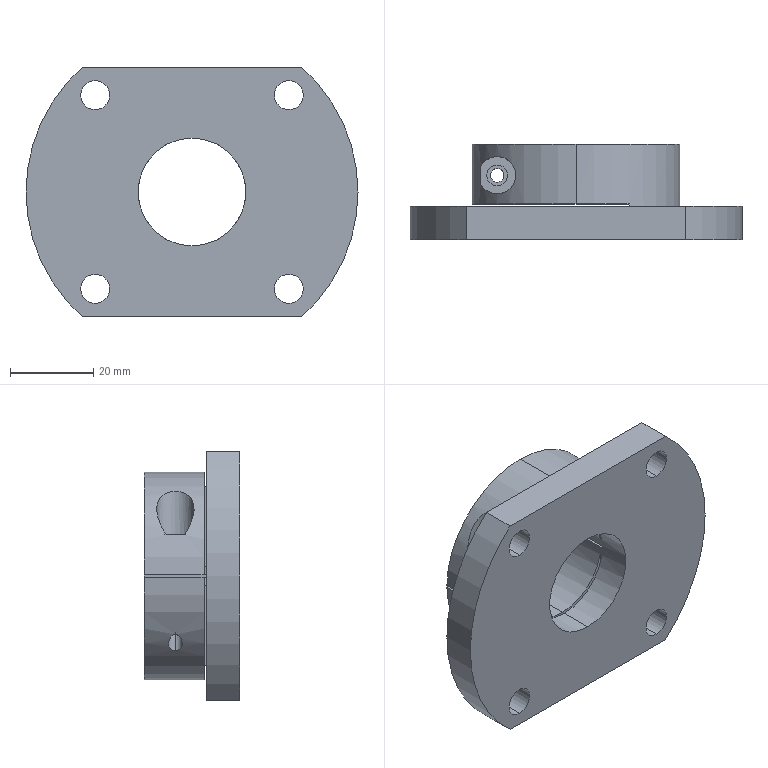Part | SolidWorks | features ICE 6, 3DProfileFeature 1, HoleWzd 1, Revolution 1 | 1 solid | 38 faces | box 80 x 23 x 60 mm | volume 48901 mm3 | cylinder 22 | plane 16 | commonest cylinder face diameters 7 x8 26 x4 50 x3 3.3 x2 5 x2 80 x2
STEP:
#1=CARTESIAN_POINT('',(-20.65,15.5,-14.092));
#2=VERTEX_POINT('',#1);
#3=CARTESIAN_POINT('',(-17.35,15.5,-17.999));
#4=VERTEX_POINT('',#3);
#5=CARTESIAN_POINT('',(-20.65,15.5,-14.092));
#6=CARTESIAN_POINT('',(-20.65,15.361,-14.092));
#7=CARTESIAN_POINT('',(-20.632,15.221,-14.119));
#8=CARTESIAN_POINT('',(-20.566,14.963,-14.214));
#9=CARTESIAN_POINT('',(-20.521,14.849,-14.28));
#10=CARTESIAN_POINT('',(-20.413,14.639,-14.434));
#11=CARTESIAN_POINT('',(-20.352,14.548,-14.52));
#12=CARTESIAN_POINT('',(-20.22,14.385,-14.702));
#13=CARTESIAN_POINT('',(-20.149,14.312,-14.8));
#14=CARTESIAN_POINT('',(-19.927,14.121,-15.098));
#15=CARTESIAN_POINT('',(-19.769,14.029,-15.305));
#16=CARTESIAN_POINT('',(-19.433,13.898,-15.73));
#17=CARTESIAN_POINT('',(-19.258,13.86,-15.944));
#18=CARTESIAN_POINT('',(-18.9,13.843,-16.367));
#19=CARTESIAN_POINT('',(-18.714,13.864,-16.579));
#20=CARTESIAN_POINT('',(-18.441,13.945,-16.881));
#21=CARTESIAN_POINT('',(-18.35,13.98,-16.979));
#22=CARTESIAN_POINT('',(-18.17,14.07,-17.171));
#23=CARTESIAN_POINT('',(-18.081,14.126,-17.266));
#24=CARTESIAN_POINT('',(-17.91,14.256,-17.442));
#25=CARTESIAN_POINT('',(-17.829,14.332,-17.526));
#26=CARTESIAN_POINT('',(-17.676,14.509,-17.68));
#27=CARTESIAN_POINT('',(-17.606,14.609,-17.75));
#28=CARTESIAN_POINT('',(-17.486,14.831,-17.867));
#29=CARTESIAN_POINT('',(-17.436,14.956,-17.916));
#30=CARTESIAN_POINT('',(-17.369,15.218,-17.981));
#31=CARTESIAN_POINT('',(-17.35,15.358,-17.999));
#32=CARTESIAN_POINT('',(-17.35,15.5,-17.999));
#33=B_SPLINE_CURVE_WITH_KNOTS('',3,(#5,#6,#7,#8,#9,#10,#11,#12,#13,#14,#15,#16,#17,#18,#19,#20,#21,#22,#23,#24,#25,#26,#27,#28,#29,#30,#31,#32),.UNSPECIFIED.,.F.,.F.,(4,2,2,2,2,2,2,2,2,2,2,2,2,4),(0.006678,0.007096,0.007513,0.007931,0.008348,0.009183,0.01002,0.01085,0.01127,0.01169,0.01211,0.01252,0.01294,0.01336),.UNSPECIFIED.);
#34=EDGE_CURVE('',#2,#4,#33,.T.);
#35=ORIENTED_EDGE('',*,*,#34,.F.);
#36=CARTESIAN_POINT('',(-20.65,15.5,-0.3));
#37=VERTEX_POINT('',#36);
#38=CARTESIAN_POINT('',(-20.65,15.5,0.3));
#39=DIRECTION('',(0.,0.,1.));
#40=VECTOR('',#39,1000.);
#41=LINE('',#38,#40);
#42=EDGE_CURVE('',#2,#37,#41,.T.);
#43=ORIENTED_EDGE('',*,*,#42,.T.);
#44=CARTESIAN_POINT('',(-17.35,15.5,-0.3));
#45=VERTEX_POINT('',#44);
#46=CARTESIAN_POINT('',(-19.,15.5,-0.3));
#47=DIRECTION('',(0.,0.,-1.));
#48=DIRECTION('',(-1.,0.,0.));
#49=AXIS2_PLACEMENT_3D('',#46,#47,#48);
#50=CIRCLE('',#49,1.65);
#51=EDGE_CURVE('',#45,#37,#50,.T.);
#52=ORIENTED_EDGE('',*,*,#51,.F.);
#53=CARTESIAN_POINT('',(-17.35,15.5,0.3));
#54=DIRECTION('',(0.,0.,1.));
#55=VECTOR('',#54,1000.);
#56=LINE('',#53,#55);
#57=EDGE_CURVE('',#4,#45,#56,.T.);
#58=ORIENTED_EDGE('',*,*,#57,.F.);
#59=EDGE_LOOP('',(#35,#43,#52,#58));
#60=FACE_OUTER_BOUND('',#59,.T.);
#61=CARTESIAN_POINT('',(-19.,15.5,0.3));
#62=DIRECTION('',(0.,0.,1.));
#63=DIRECTION('',(1.,0.,0.));
#64=AXIS2_PLACEMENT_3D('',#61,#62,#63);
#65=CYLINDRICAL_SURFACE('',#64,1.65);
#66=ADVANCED_FACE('',(#60),#65,.F.);
#67=CARTESIAN_POINT('',(-16.5,15.5,0.3));
#68=VERTEX_POINT('',#67);
#69=CARTESIAN_POINT('',(-21.5,15.5,0.3));
#70=VERTEX_POINT('',#69);
#71=CARTESIAN_POINT('',(-19.,15.5,0.3));
#72=DIRECTION('',(0.,0.,-1.));
#73=DIRECTION('',(1.,0.,0.));
#74=AXIS2_PLACEMENT_3D('',#71,#72,#73);
#75=CIRCLE('',#74,2.5);
#76=EDGE_CURVE('',#68,#70,#75,.T.);
#77=ORIENTED_EDGE('',*,*,#76,.T.);
#78=CARTESIAN_POINT('',(-21.5,15.5,10.));
#79=VERTEX_POINT('',#78);
#80=CARTESIAN_POINT('',(-21.5,15.5,-30.001));
#81=DIRECTION('',(0.,0.,1.));
#82=VECTOR('',#81,1000.);
#83=LINE('',#80,#82);
#84=EDGE_CURVE('',#70,#79,#83,.T.);
#85=ORIENTED_EDGE('',*,*,#84,.T.);
#86=CARTESIAN_POINT('',(-16.5,15.5,10.));
#87=VERTEX_POINT('',#86);
#88=CARTESIAN_POINT('',(-19.,15.5,10.));
#89=DIRECTION('',(0.,0.,1.));
#90=DIRECTION('',(1.,0.,0.));
#91=AXIS2_PLACEMENT_3D('',#88,#89,#90);
#92=CIRCLE('',#91,2.5);
#93=EDGE_CURVE('',#79,#87,#92,.T.);
#94=ORIENTED_EDGE('',*,*,#93,.T.);
#95=CARTESIAN_POINT('',(-16.5,15.5,-30.001));
#96=DIRECTION('',(0.,0.,1.));
#97=VECTOR('',#96,1000.);
#98=LINE('',#95,#97);
#99=EDGE_CURVE('',#68,#87,#98,.T.);
#100=ORIENTED_EDGE('',*,*,#99,.F.);
#101=EDGE_LOOP('',(#77,#85,#94,#100));
#102=FACE_OUTER_BOUND('',#101,.T.);
#103=CARTESIAN_POINT('',(-19.,15.5,-30.001));
#104=DIRECTION('',(0.,0.,1.));
#105=DIRECTION('',(1.,0.,0.));
#106=AXIS2_PLACEMENT_3D('',#103,#104,#105);
#107=CYLINDRICAL_SURFACE('',#106,2.5);
#108=ADVANCED_FACE('',(#102),#107,.F.);
#109=CARTESIAN_POINT('',(23.335,0.,-26.835));
#110=VERTEX_POINT('',#109);
#111=CARTESIAN_POINT('',(23.335,0.,-19.835));
#112=VERTEX_POINT('',#111);
#113=CARTESIAN_POINT('',(23.335,0.,-23.335));
#114=DIRECTION('',(0.,1.,0.));
#115=DIRECTION('',(0.,0.,1.));
#116=AXIS2_PLACEMENT_3D('',#113,#114,#115);
#117=CIRCLE('',#116,3.5);
#118=EDGE_CURVE('',#110,#112,#117,.T.);
#119=ORIENTED_EDGE('',*,*,#118,.F.);
#120=CARTESIAN_POINT('',(23.335,8.,-26.835));
#121=VERTEX_POINT('',#120);
#122=CARTESIAN_POINT('',(23.335,-22.,-26.835));
#123=DIRECTION('',(0.,1.,0.));
#124=VECTOR('',#123,1000.);
#125=LINE('',#122,#124);
#126=EDGE_CURVE('',#110,#121,#125,.T.);
#127=ORIENTED_EDGE('',*,*,#126,.T.);
#128=CARTESIAN_POINT('',(23.335,8.,-19.835));
#129=VERTEX_POINT('',#128);
#130=CARTESIAN_POINT('',(23.335,8.,-23.335));
#131=DIRECTION('',(0.,1.,0.));
#132=DIRECTION('',(0.,0.,1.));
#133=AXIS2_PLACEMENT_3D('',#130,#131,#132);
#134=CIRCLE('',#133,3.5);
#135=EDGE_CURVE('',#121,#129,#134,.T.);
#136=ORIENTED_EDGE('',*,*,#135,.T.);
#137=CARTESIAN_POINT('',(23.335,-22.,-19.835));
#138=DIRECTION('',(0.,1.,0.));
#139=VECTOR('',#138,1000.);
#140=LINE('',#137,#139);
#141=EDGE_CURVE('',#112,#129,#140,.T.);
#142=ORIENTED_EDGE('',*,*,#141,.F.);
#143=EDGE_LOOP('',(#119,#127,#136,#142));
#144=FACE_OUTER_BOUND('',#143,.T.);
#145=CARTESIAN_POINT('',(23.335,-22.,-23.335));
#146=DIRECTION('',(0.,1.,0.));
#147=DIRECTION('',(0.,0.,1.));
#148=AXIS2_PLACEMENT_3D('',#145,#146,#147);
#149=CYLINDRICAL_SURFACE('',#148,3.5);
#150=ADVANCED_FACE('',(#144),#149,.F.);
#151=CARTESIAN_POINT('',(23.335,0.,19.835));
#152=VERTEX_POINT('',#151);
#153=CARTESIAN_POINT('',(23.335,0.,26.835));
#154=VERTEX_POINT('',#153);
#155=CARTESIAN_POINT('',(23.335,0.,23.335));
#156=DIRECTION('',(0.,1.,0.));
#157=DIRECTION('',(0.,0.,1.));
#158=AXIS2_PLACEMENT_3D('',#155,#156,#157);
#159=CIRCLE('',#158,3.5);
#160=EDGE_CURVE('',#152,#154,#159,.T.);
#161=ORIENTED_EDGE('',*,*,#160,.F.);
#162=CARTESIAN_POINT('',(23.335,8.,19.835));
#163=VERTEX_POINT('',#162);
#164=CARTESIAN_POINT('',(23.335,-22.,19.835));
#165=DIRECTION('',(0.,1.,0.));
#166=VECTOR('',#165,1000.);
#167=LINE('',#164,#166);
#168=EDGE_CURVE('',#152,#163,#167,.T.);
#169=ORIENTED_EDGE('',*,*,#168,.T.);
#170=CARTESIAN_POINT('',(23.335,8.,26.835));
#171=VERTEX_POINT('',#170);
#172=CARTESIAN_POINT('',(23.335,8.,23.335));
#173=DIRECTION('',(0.,1.,0.));
#174=DIRECTION('',(0.,0.,1.));
#175=AXIS2_PLACEMENT_3D('',#172,#173,#174);
#176=CIRCLE('',#175,3.5);
#177=EDGE_CURVE('',#163,#171,#176,.T.);
#178=ORIENTED_EDGE('',*,*,#177,.T.);
#179=CARTESIAN_POINT('',(23.335,-22.,26.835));
#180=DIRECTION('',(0.,1.,0.));
#181=VECTOR('',#180,1000.);
#182=LINE('',#179,#181);
#183=EDGE_CURVE('',#154,#171,#182,.T.);
#184=ORIENTED_EDGE('',*,*,#183,.F.);
#185=EDGE_LOOP('',(#161,#169,#178,#184));
#186=FACE_OUTER_BOUND('',#185,.T.);
#187=CARTESIAN_POINT('',(23.335,-22.,23.335));
#188=DIRECTION('',(0.,1.,0.));
#189=DIRECTION('',(0.,0.,1.));
#190=AXIS2_PLACEMENT_3D('',#187,#188,#189);
#191=CYLINDRICAL_SURFACE('',#190,3.5);
#192=ADVANCED_FACE('',(#186),#191,.F.);
#193=CARTESIAN_POINT('',(-23.335,0.,19.835));
#194=VERTEX_POINT('',#193);
#195=CARTESIAN_POINT('',(-23.335,0.,26.835));
#196=VERTEX_POINT('',#195);
#197=CARTESIAN_POINT('',(-23.335,0.,23.335));
#198=DIRECTION('',(0.,1.,0.));
#199=DIRECTION('',(0.,0.,1.));
#200=AXIS2_PLACEMENT_3D('',#197,#198,#199);
#201=CIRCLE('',#200,3.5);
#202=EDGE_CURVE('',#194,#196,#201,.T.);
#203=ORIENTED_EDGE('',*,*,#202,.F.);
#204=CARTESIAN_POINT('',(-23.335,8.,19.835));
#205=VERTEX_POINT('',#204);
#206=CARTESIAN_POINT('',(-23.335,-22.,19.835));
#207=DIRECTION('',(0.,1.,0.));
#208=VECTOR('',#207,1000.);
#209=LINE('',#206,#208);
#210=EDGE_CURVE('',#194,#205,#209,.T.);
#211=ORIENTED_EDGE('',*,*,#210,.T.);
#212=CARTESIAN_POINT('',(-23.335,8.,26.835));
#213=VERTEX_POINT('',#212);
#214=CARTESIAN_POINT('',(-23.335,8.,23.335));
#215=DIRECTION('',(0.,1.,0.));
#216=DIRECTION('',(0.,0.,1.));
#217=AXIS2_PLACEMENT_3D('',#214,#215,#216);
#218=CIRCLE('',#217,3.5);
#219=EDGE_CURVE('',#205,#213,#218,.T.);
#220=ORIENTED_EDGE('',*,*,#219,.T.);
#221=CARTESIAN_POINT('',(-23.335,-22.,26.835));
#222=DIRECTION('',(0.,1.,0.));
#223=VECTOR('',#222,1000.);
#224=LINE('',#221,#223);
#225=EDGE_CURVE('',#196,#213,#224,.T.);
#226=ORIENTED_EDGE('',*,*,#225,.F.);
#227=EDGE_LOOP('',(#203,#211,#220,#226));
#228=FACE_OUTER_BOUND('',#227,.T.);
#229=CARTESIAN_POINT('',(-23.335,-22.,23.335));
#230=DIRECTION('',(0.,1.,0.));
#231=DIRECTION('',(0.,0.,1.));
#232=AXIS2_PLACEMENT_3D('',#229,#230,#231);
#233=CYLINDRICAL_SURFACE('',#232,3.5);
#234=ADVANCED_FACE('',(#228),#233,.F.);
#235=CARTESIAN_POINT('',(-23.335,0.,-26.835));
#236=VERTEX_POINT('',#235);
#237=CARTESIAN_POINT('',(-23.335,0.,-19.835));
#238=VERTEX_POINT('',#237);
#239=CARTESIAN_POINT('',(-23.335,0.,-23.335));
#240=DIRECTION('',(0.,1.,0.));
#241=DIRECTION('',(0.,0.,1.));
#242=AXIS2_PLACEMENT_3D('',#239,#240,#241);
#243=CIRCLE('',#242,3.5);
#244=EDGE_CURVE('',#236,#238,#243,.T.);
#245=ORIENTED_EDGE('',*,*,#244,.F.);
#246=CARTESIAN_POINT('',(-23.335,8.,-26.835));
#247=VERTEX_POINT('',#246);
#248=CARTESIAN_POINT('',(-23.335,-22.,-26.835));
#249=DIRECTION('',(0.,1.,0.));
#250=VECTOR('',#249,1000.);
#251=LINE('',#248,#250);
#252=EDGE_CURVE('',#236,#247,#251,.T.);
#253=ORIENTED_EDGE('',*,*,#252,.T.);
#254=CARTESIAN_POINT('',(-23.335,8.,-19.835));
#255=VERTEX_POINT('',#254);
#256=CARTESIAN_POINT('',(-23.335,8.,-23.335));
#257=DIRECTION('',(0.,1.,0.));
#258=DIRECTION('',(0.,0.,1.));
#259=AXIS2_PLACEMENT_3D('',#256,#257,#258);
#260=CIRCLE('',#259,3.5);
#261=EDGE_CURVE('',#247,#255,#260,.T.);
#262=ORIENTED_EDGE('',*,*,#261,.T.);
#263=CARTESIAN_POINT('',(-23.335,-22.,-19.835));
#264=DIRECTION('',(0.,1.,0.));
#265=VECTOR('',#264,1000.);
#266=LINE('',#263,#265);
#267=EDGE_CURVE('',#238,#255,#266,.T.);
#268=ORIENTED_EDGE('',*,*,#267,.F.);
#269=EDGE_LOOP('',(#245,#253,#262,#268));
#270=FACE_OUTER_BOUND('',#269,.T.);
#271=CARTESIAN_POINT('',(-23.335,-22.,-23.335));
#272=DIRECTION('',(0.,1.,0.));
#273=DIRECTION('',(0.,0.,1.));
#274=AXIS2_PLACEMENT_3D('',#271,#272,#273);
#275=CYLINDRICAL_SURFACE('',#274,3.5);
#276=ADVANCED_FACE('',(#270),#275,.F.);
#277=CARTESIAN_POINT('',(0.,23.,13.));
#278=VERTEX_POINT('',#277);
#279=CARTESIAN_POINT('',(-12.997,23.,0.3));
#280=VERTEX_POINT('',#279);
#281=CARTESIAN_POINT('',(0.,23.,0.));
#282=DIRECTION('',(0.,-1.,0.));
#283=DIRECTION('',(0.,0.,-1.));
#284=AXIS2_PLACEMENT_3D('',#281,#282,#283);
#285=CIRCLE('',#284,13.);
#286=EDGE_CURVE('',#278,#280,#285,.T.);
#287=ORIENTED_EDGE('',*,*,#286,.F.);
#288=CARTESIAN_POINT('',(0.,8.6,13.));
#289=VERTEX_POINT('',#288);
#290=CARTESIAN_POINT('',(0.,0.,13.));
#291=DIRECTION('',(0.,-1.,0.));
#292=VECTOR('',#291,1000.);
#293=LINE('',#290,#292);
#294=EDGE_CURVE('',#278,#289,#293,.T.);
#295=ORIENTED_EDGE('',*,*,#294,.T.);
#296=CARTESIAN_POINT('',(-12.997,8.6,0.3));
#297=VERTEX_POINT('',#296);
#298=CARTESIAN_POINT('',(0.,8.6,0.));
#299=DIRECTION('',(0.,-1.,0.));
#300=DIRECTION('',(-1.,0.,0.));
#301=AXIS2_PLACEMENT_3D('',#298,#299,#300);
#302=CIRCLE('',#301,13.);
#303=EDGE_CURVE('',#289,#297,#302,.T.);
#304=ORIENTED_EDGE('',*,*,#303,.T.);
#305=CARTESIAN_POINT('',(-12.997,0.,0.3));
#306=DIRECTION('',(0.,1.,0.));
#307=VECTOR('',#306,1000.);
#308=LINE('',#305,#307);
#309=EDGE_CURVE('',#297,#280,#308,.T.);
#310=ORIENTED_EDGE('',*,*,#309,.T.);
#311=EDGE_LOOP('',(#287,#295,#304,#310));
#312=FACE_OUTER_BOUND('',#311,.T.);
#313=CARTESIAN_POINT('',(0.,0.,0.));
#314=DIRECTION('',(0.,-1.,0.));
#315=DIRECTION('',(0.,0.,-1.));
#316=AXIS2_PLACEMENT_3D('',#313,#314,#315);
#317=CYLINDRICAL_SURFACE('',#316,13.);
#318=ADVANCED_FACE('',(#312),#317,.F.);
#319=CARTESIAN_POINT('',(0.,8.,-13.));
#320=VERTEX_POINT('',#319);
#321=CARTESIAN_POINT('',(0.,8.,13.));
#322=VERTEX_POINT('',#321);
#323=CARTESIAN_POINT('',(0.,8.,0.));
#324=DIRECTION('',(0.,1.,0.));
#325=DIRECTION('',(0.,0.,-1.));
#326=AXIS2_PLACEMENT_3D('',#323,#324,#325);
#327=CIRCLE('',#326,13.);
#328=EDGE_CURVE('',#320,#322,#327,.T.);
#329=ORIENTED_EDGE('',*,*,#328,.T.);
#330=CARTESIAN_POINT('',(0.,0.,13.));
#331=VERTEX_POINT('',#330);
#332=CARTESIAN_POINT('',(0.,0.,13.));
#333=DIRECTION('',(0.,-1.,0.));
#334=VECTOR('',#333,1000.);
#335=LINE('',#332,#334);
#336=EDGE_CURVE('',#322,#331,#335,.T.);
#337=ORIENTED_EDGE('',*,*,#336,.T.);
#338=CARTESIAN_POINT('',(0.,0.,-13.));
#339=VERTEX_POINT('',#338);
#340=CARTESIAN_POINT('',(0.,0.,0.));
#341=DIRECTION('',(0.,-1.,0.));
#342=DIRECTION('',(0.,0.,-1.));
#343=AXIS2_PLACEMENT_3D('',#340,#341,#342);
#344=CIRCLE('',#343,13.);
#345=EDGE_CURVE('',#331,#339,#344,.T.);
#346=ORIENTED_EDGE('',*,*,#345,.T.);
#347=CARTESIAN_POINT('',(0.,0.,-13.));
#348=DIRECTION('',(0.,-1.,0.));
#349=VECTOR('',#348,1000.);
#350=LINE('',#347,#349);
#351=EDGE_CURVE('',#320,#339,#350,.T.);
#352=ORIENTED_EDGE('',*,*,#351,.F.);
#353=EDGE_LOOP('',(#329,#337,#346,#352));
#354=FACE_OUTER_BOUND('',#353,.T.);
#355=CARTESIAN_POINT('',(0.,0.,0.));
#356=DIRECTION('',(0.,-1.,0.));
#357=DIRECTION('',(0.,0.,-1.));
#358=AXIS2_PLACEMENT_3D('',#355,#356,#357);
#359=CYLINDRICAL_SURFACE('',#358,13.);
#360=ADVANCED_FACE('',(#354),#359,.F.);
#361=ORIENTED_EDGE('',*,*,#294,.F.);
#362=CARTESIAN_POINT('',(12.997,23.,0.3));
#363=VERTEX_POINT('',#362);
#364=CARTESIAN_POINT('',(0.,23.,0.));
#365=DIRECTION('',(0.,-1.,0.));
#366=DIRECTION('',(0.,0.,-1.));
#367=AXIS2_PLACEMENT_3D('',#364,#365,#366);
#368=CIRCLE('',#367,13.);
#369=EDGE_CURVE('',#363,#278,#368,.T.);
#370=ORIENTED_EDGE('',*,*,#369,.F.);
#371=CARTESIAN_POINT('',(12.997,8.,0.3));
#372=VERTEX_POINT('',#371);
#373=CARTESIAN_POINT('',(12.997,0.,0.3));
#374=DIRECTION('',(0.,-1.,0.));
#375=VECTOR('',#374,1000.);
#376=LINE('',#373,#375);
#377=EDGE_CURVE('',#363,#372,#376,.T.);
#378=ORIENTED_EDGE('',*,*,#377,.T.);
#379=CARTESIAN_POINT('',(12.997,8.,-0.3));
#380=VERTEX_POINT('',#379);
#381=CARTESIAN_POINT('',(0.,8.,0.));
#382=DIRECTION('',(0.,-1.,0.));
#383=DIRECTION('',(0.,0.,1.));
#384=AXIS2_PLACEMENT_3D('',#381,#382,#383);
#385=CIRCLE('',#384,13.);
#386=EDGE_CURVE('',#380,#372,#385,.T.);
#387=ORIENTED_EDGE('',*,*,#386,.F.);
#388=CARTESIAN_POINT('',(12.997,23.,-0.3));
#389=VERTEX_POINT('',#388);
#390=CARTESIAN_POINT('',(12.997,0.,-0.3));
#391=DIRECTION('',(0.,1.,0.));
#392=VECTOR('',#391,1000.);
#393=LINE('',#390,#392);
#394=EDGE_CURVE('',#380,#389,#393,.T.);
#395=ORIENTED_EDGE('',*,*,#394,.T.);
#396=CARTESIAN_POINT('',(0.,23.,-13.));
#397=VERTEX_POINT('',#396);
#398=CARTESIAN_POINT('',(0.,23.,0.));
#399=DIRECTION('',(0.,-1.,0.));
#400=DIRECTION('',(0.,0.,-1.));
#401=AXIS2_PLACEMENT_3D('',#398,#399,#400);
#402=CIRCLE('',#401,13.);
#403=EDGE_CURVE('',#397,#389,#402,.T.);
#404=ORIENTED_EDGE('',*,*,#403,.F.);
#405=CARTESIAN_POINT('',(0.,8.6,-13.));
#406=VERTEX_POINT('',#405);
#407=CARTESIAN_POINT('',(0.,0.,-13.));
#408=DIRECTION('',(0.,-1.,0.));
#409=VECTOR('',#408,1000.);
#410=LINE('',#407,#409);
#411=EDGE_CURVE('',#397,#406,#410,.T.);
#412=ORIENTED_EDGE('',*,*,#411,.T.);
#413=CARTESIAN_POINT('',(12.79,8.6,-2.326));
#414=VERTEX_POINT('',#413);
#415=CARTESIAN_POINT('',(0.,8.6,0.));
#416=DIRECTION('',(0.,-1.,0.));
#417=DIRECTION('',(-1.,0.,0.));
#418=AXIS2_PLACEMENT_3D('',#415,#416,#417);
#419=CIRCLE('',#418,13.);
#420=EDGE_CURVE('',#406,#414,#419,.T.);
#421=ORIENTED_EDGE('',*,*,#420,.T.);
#422=CARTESIAN_POINT('',(12.79,8.,-2.326));
#423=VERTEX_POINT('',#422);
#424=CARTESIAN_POINT('',(12.79,0.,-2.326));
#425=DIRECTION('',(0.,-1.,0.));
#426=VECTOR('',#425,1000.);
#427=LINE('',#424,#426);
#428=EDGE_CURVE('',#414,#423,#427,.T.);
#429=ORIENTED_EDGE('',*,*,#428,.T.);
#430=CARTESIAN_POINT('',(0.,8.,0.));
#431=DIRECTION('',(0.,1.,0.));
#432=DIRECTION('',(0.,0.,-1.));
#433=AXIS2_PLACEMENT_3D('',#430,#431,#432);
#434=CIRCLE('',#433,13.);
#435=EDGE_CURVE('',#423,#320,#434,.T.);
#436=ORIENTED_EDGE('',*,*,#435,.T.);
#437=ORIENTED_EDGE('',*,*,#351,.T.);
#438=CARTESIAN_POINT('',(0.,0.,0.));
#439=DIRECTION('',(0.,-1.,0.));
#440=DIRECTION('',(0.,0.,-1.));
#441=AXIS2_PLACEMENT_3D('',#438,#439,#440);
#442=CIRCLE('',#441,13.);
#443=EDGE_CURVE('',#339,#331,#442,.T.);
#444=ORIENTED_EDGE('',*,*,#443,.T.);
#445=ORIENTED_EDGE('',*,*,#336,.F.);
#446=CARTESIAN_POINT('',(12.79,8.,2.326));
#447=VERTEX_POINT('',#446);
#448=CARTESIAN_POINT('',(0.,8.,0.));
#449=DIRECTION('',(0.,1.,0.));
#450=DIRECTION('',(0.,0.,-1.));
#451=AXIS2_PLACEMENT_3D('',#448,#449,#450);
#452=CIRCLE('',#451,13.);
#453=EDGE_CURVE('',#322,#447,#452,.T.);
#454=ORIENTED_EDGE('',*,*,#453,.T.);
#455=CARTESIAN_POINT('',(12.79,8.6,2.326));
#456=VERTEX_POINT('',#455);
#457=CARTESIAN_POINT('',(12.79,0.,2.326));
#458=DIRECTION('',(0.,1.,0.));
#459=VECTOR('',#458,1000.);
#460=LINE('',#457,#459);
#461=EDGE_CURVE('',#447,#456,#460,.T.);
#462=ORIENTED_EDGE('',*,*,#461,.T.);
#463=CARTESIAN_POINT('',(0.,8.6,0.));
#464=DIRECTION('',(0.,-1.,0.));
#465=DIRECTION('',(-1.,0.,0.));
#466=AXIS2_PLACEMENT_3D('',#463,#464,#465);
#467=CIRCLE('',#466,13.);
#468=EDGE_CURVE('',#456,#289,#467,.T.);
#469=ORIENTED_EDGE('',*,*,#468,.T.);
#470=EDGE_LOOP('',(#361,#370,#378,#387,#395,#404,#412,#421,#429,#436,#437,#444,#445,#454,#462,#469));
#471=FACE_OUTER_BOUND('',#470,.T.);
#472=CARTESIAN_POINT('',(0.,0.,0.));
#473=DIRECTION('',(0.,-1.,0.));
#474=DIRECTION('',(0.,0.,-1.));
#475=AXIS2_PLACEMENT_3D('',#472,#473,#474);
#476=CYLINDRICAL_SURFACE('',#475,13.);
#477=ADVANCED_FACE('',(#471),#476,.F.);
#478=CARTESIAN_POINT('',(0.,23.,-25.));
#479=VERTEX_POINT('',#478);
#480=CARTESIAN_POINT('',(0.,23.,25.));
#481=VERTEX_POINT('',#480);
#482=CARTESIAN_POINT('',(0.,23.,0.));
#483=DIRECTION('',(0.,-1.,0.));
#484=DIRECTION('',(0.,0.,-1.));
#485=AXIS2_PLACEMENT_3D('',#482,#483,#484);
#486=CIRCLE('',#485,25.);
#487=EDGE_CURVE('',#479,#481,#486,.T.);
#488=ORIENTED_EDGE('',*,*,#487,.T.);
#489=CARTESIAN_POINT('',(0.,8.6,25.));
#490=VERTEX_POINT('',#489);
#491=CARTESIAN_POINT('',(0.,0.,25.));
#492=DIRECTION('',(0.,-1.,0.));
#493=VECTOR('',#492,1000.);
#494=LINE('',#491,#493);
#495=EDGE_CURVE('',#481,#490,#494,.T.);
#496=ORIENTED_EDGE('',*,*,#495,.T.);
#497=CARTESIAN_POINT('',(12.79,8.6,21.48));
#498=VERTEX_POINT('',#497);
#499=CARTESIAN_POINT('',(0.,8.6,0.));
#500=DIRECTION('',(0.,1.,0.));
#501=DIRECTION('',(-1.,0.,0.));
#502=AXIS2_PLACEMENT_3D('',#499,#500,#501);
#503=CIRCLE('',#502,25.);
#504=EDGE_CURVE('',#490,#498,#503,.T.);
#505=ORIENTED_EDGE('',*,*,#504,.T.);
#506=CARTESIAN_POINT('',(12.79,8.,21.48));
#507=VERTEX_POINT('',#506);
#508=CARTESIAN_POINT('',(12.79,0.,21.48));
#509=DIRECTION('',(0.,-1.,0.));
#510=VECTOR('',#509,1000.);
#511=LINE('',#508,#510);
#512=EDGE_CURVE('',#498,#507,#511,.T.);
#513=ORIENTED_EDGE('',*,*,#512,.T.);
#514=CARTESIAN_POINT('',(12.79,8.,-21.48));
#515=VERTEX_POINT('',#514);
#516=CARTESIAN_POINT('',(0.,8.,0.));
#517=DIRECTION('',(0.,-1.,0.));
#518=DIRECTION('',(0.,0.,-1.));
#519=AXIS2_PLACEMENT_3D('',#516,#517,#518);
#520=CIRCLE('',#519,25.);
#521=EDGE_CURVE('',#515,#507,#520,.T.);
#522=ORIENTED_EDGE('',*,*,#521,.F.);
#523=CARTESIAN_POINT('',(12.79,8.6,-21.48));
#524=VERTEX_POINT('',#523);
#525=CARTESIAN_POINT('',(12.79,0.,-21.48));
#526=DIRECTION('',(0.,1.,0.));
#527=VECTOR('',#526,1000.);
#528=LINE('',#525,#527);
#529=EDGE_CURVE('',#515,#524,#528,.T.);
#530=ORIENTED_EDGE('',*,*,#529,.T.);
#531=CARTESIAN_POINT('',(0.,8.6,-25.));
#532=VERTEX_POINT('',#531);
#533=CARTESIAN_POINT('',(0.,8.6,0.));
#534=DIRECTION('',(0.,1.,0.));
#535=DIRECTION('',(-1.,0.,0.));
#536=AXIS2_PLACEMENT_3D('',#533,#534,#535);
#537=CIRCLE('',#536,25.);
#538=EDGE_CURVE('',#524,#532,#537,.T.);
#539=ORIENTED_EDGE('',*,*,#538,.T.);
#540=CARTESIAN_POINT('',(0.,0.,-25.));
#541=DIRECTION('',(0.,-1.,0.));
#542=VECTOR('',#541,1000.);
#543=LINE('',#540,#542);
#544=EDGE_CURVE('',#479,#532,#543,.T.);
#545=ORIENTED_EDGE('',*,*,#544,.F.);
#546=EDGE_LOOP('',(#488,#496,#505,#513,#522,#530,#539,#545));
#547=FACE_OUTER_BOUND('',#546,.T.);
#548=CARTESIAN_POINT('',(0.,0.,0.));
#549=DIRECTION('',(0.,-1.,0.));
#550=DIRECTION('',(0.,0.,-1.));
#551=AXIS2_PLACEMENT_3D('',#548,#549,#550);
#552=CYLINDRICAL_SURFACE('',#551,25.);
#553=ADVANCED_FACE('',(#547),#552,.T.);
#554=CARTESIAN_POINT('',(-17.35,15.5,-17.999));
#555=CARTESIAN_POINT('',(-17.35,15.783,-17.999));
#556=CARTESIAN_POINT('',(-17.425,16.054,-17.928));
#557=CARTESIAN_POINT('',(-17.666,16.504,-17.69));
#558=CARTESIAN_POINT('',(-17.825,16.679,-17.53));
#559=CARTESIAN_POINT('',(-18.081,16.875,-17.265));
#560=CARTESIAN_POINT('',(-18.169,16.929,-17.172));
#561=CARTESIAN_POINT('',(-18.349,17.019,-16.98));
#562=CARTESIAN_POINT('',(-18.441,17.055,-16.88));
#563=CARTESIAN_POINT('',(-18.716,17.137,-16.576));
#564=CARTESIAN_POINT('',(-18.898,17.157,-16.369));
#565=CARTESIAN_POINT('',(-19.258,17.14,-15.944));
#566=CARTESIAN_POINT('',(-19.434,17.102,-15.729));
#567=CARTESIAN_POINT('',(-19.767,16.972,-15.308));
#568=CARTESIAN_POINT('',(-19.929,16.878,-15.096));
#569=CARTESIAN_POINT('',(-20.15,16.687,-14.798));
#570=CARTESIAN_POINT('',(-20.221,16.615,-14.702));
#571=CARTESIAN_POINT('',(-20.353,16.451,-14.518));
#572=CARTESIAN_POINT('',(-20.414,16.358,-14.432));
#573=CARTESIAN_POINT('',(-20.521,16.151,-14.28));
#574=CARTESIAN_POINT('',(-20.567,16.033,-14.213));
#575=CARTESIAN_POINT('',(-20.632,15.779,-14.119));
#576=CARTESIAN_POINT('',(-20.65,15.639,-14.092));
#577=CARTESIAN_POINT('',(-20.65,15.5,-14.092));
#578=B_SPLINE_CURVE_WITH_KNOTS('',3,(#554,#555,#556,#557,#558,#559,#560,#561,#562,#563,#564,#565,#566,#567,#568,#569,#570,#571,#572,#573,#574,#575,#576,#577),.UNSPECIFIED.,.F.,.F.,(4,2,2,2,2,2,2,2,2,2,2,4),(0.,0.0008348,0.00167,0.002087,0.002504,0.003339,0.004174,0.005009,0.005426,0.005843,0.006261,0.006678),.UNSPECIFIED.);
#579=EDGE_CURVE('',#4,#2,#578,.T.);
#580=ORIENTED_EDGE('',*,*,#579,.T.);
#581=ORIENTED_EDGE('',*,*,#34,.T.);
#582=EDGE_LOOP('',(#580,#581));
#583=FACE_BOUND('',#582,.T.);
#584=CARTESIAN_POINT('',(-24.998,23.,-0.3));
#585=VERTEX_POINT('',#584);
#586=CARTESIAN_POINT('',(0.,23.,0.));
#587=DIRECTION('',(0.,-1.,0.));
#588=DIRECTION('',(0.,0.,-1.));
#589=AXIS2_PLACEMENT_3D('',#586,#587,#588);
#590=CIRCLE('',#589,25.);
#591=EDGE_CURVE('',#585,#479,#590,.T.);
#592=ORIENTED_EDGE('',*,*,#591,.T.);
#593=ORIENTED_EDGE('',*,*,#544,.T.);
#594=CARTESIAN_POINT('',(-24.998,8.6,-0.3));
#595=VERTEX_POINT('',#594);
#596=CARTESIAN_POINT('',(0.,8.6,0.));
#597=DIRECTION('',(0.,1.,0.));
#598=DIRECTION('',(-1.,0.,0.));
#599=AXIS2_PLACEMENT_3D('',#596,#597,#598);
#600=CIRCLE('',#599,25.);
#601=EDGE_CURVE('',#532,#595,#600,.T.);
#602=ORIENTED_EDGE('',*,*,#601,.T.);
#603=CARTESIAN_POINT('',(-24.998,0.,-0.3));
#604=DIRECTION('',(0.,1.,0.));
#605=VECTOR('',#604,1000.);
#606=LINE('',#603,#605);
#607=EDGE_CURVE('',#595,#585,#606,.T.);
#608=ORIENTED_EDGE('',*,*,#607,.T.);
#609=EDGE_LOOP('',(#592,#593,#602,#608));
#610=FACE_OUTER_BOUND('',#609,.T.);
#611=CARTESIAN_POINT('',(0.,0.,0.));
#612=DIRECTION('',(0.,-1.,0.));
#613=DIRECTION('',(0.,0.,-1.));
#614=AXIS2_PLACEMENT_3D('',#611,#612,#613);
#615=CYLINDRICAL_SURFACE('',#614,25.);
#616=ADVANCED_FACE('',(#583,#610),#615,.T.);
#617=ORIENTED_EDGE('',*,*,#495,.F.);
#618=CARTESIAN_POINT('',(-24.998,23.,0.3));
#619=VERTEX_POINT('',#618);
#620=CARTESIAN_POINT('',(0.,23.,0.));
#621=DIRECTION('',(0.,-1.,0.));
#622=DIRECTION('',(0.,0.,-1.));
#623=AXIS2_PLACEMENT_3D('',#620,#621,#622);
#624=CIRCLE('',#623,25.);
#625=EDGE_CURVE('',#481,#619,#624,.T.);
#626=ORIENTED_EDGE('',*,*,#625,.T.);
#627=CARTESIAN_POINT('',(-24.998,8.6,0.3));
#628=VERTEX_POINT('',#627);
#629=CARTESIAN_POINT('',(-24.998,0.,0.3));
#630=DIRECTION('',(0.,-1.,0.));
#631=VECTOR('',#630,1000.);
#632=LINE('',#629,#631);
#633=EDGE_CURVE('',#619,#628,#632,.T.);
#634=ORIENTED_EDGE('',*,*,#633,.T.);
#635=CARTESIAN_POINT('',(0.,8.6,0.));
#636=DIRECTION('',(0.,1.,0.));
#637=DIRECTION('',(-1.,0.,0.));
#638=AXIS2_PLACEMENT_3D('',#635,#636,#637);
#639=CIRCLE('',#638,25.);
#640=EDGE_CURVE('',#628,#490,#639,.T.);
#641=ORIENTED_EDGE('',*,*,#640,.T.);
#642=EDGE_LOOP('',(#617,#626,#634,#641));
#643=FACE_OUTER_BOUND('',#642,.T.);
#644=CARTESIAN_POINT('',(-22.913,13.278,10.));
#645=VERTEX_POINT('',#644);
#646=CARTESIAN_POINT('',(-22.913,17.722,10.));
#647=VERTEX_POINT('',#646);
#648=CARTESIAN_POINT('',(-22.913,13.278,10.));
#649=CARTESIAN_POINT('',(-22.801,13.08,10.256));
#650=CARTESIAN_POINT('',(-22.681,12.903,10.52));
#651=CARTESIAN_POINT('',(-22.426,12.575,11.053));
#652=CARTESIAN_POINT('',(-22.291,12.424,11.323));
#653=CARTESIAN_POINT('',(-22.006,12.145,11.867));
#654=CARTESIAN_POINT('',(-21.856,12.017,12.142));
#655=CARTESIAN_POINT('',(-21.54,11.78,12.694));
#656=CARTESIAN_POINT('',(-21.374,11.672,12.972));
#657=CARTESIAN_POINT('',(-20.857,11.382,13.799));
#658=CARTESIAN_POINT('',(-20.487,11.233,14.343));
#659=CARTESIAN_POINT('',(-19.891,11.084,15.147));
#660=CARTESIAN_POINT('',(-19.686,11.047,15.414));
#661=CARTESIAN_POINT('',(-19.26,11.002,15.943));
#662=CARTESIAN_POINT('',(-19.04,10.995,16.205));
#663=CARTESIAN_POINT('',(-18.594,11.013,16.714));
#664=CARTESIAN_POINT('',(-18.367,11.039,16.964));
#665=CARTESIAN_POINT('',(-17.905,11.129,17.451));
#666=CARTESIAN_POINT('',(-17.669,11.194,17.689));
#667=CARTESIAN_POINT('',(-17.196,11.37,18.149));
#668=CARTESIAN_POINT('',(-16.962,11.479,18.368));
#669=CARTESIAN_POINT('',(-16.5,11.749,18.784));
#670=CARTESIAN_POINT('',(-16.271,11.91,18.983));
#671=CARTESIAN_POINT('',(-15.835,12.288,19.348));
#672=CARTESIAN_POINT('',(-15.63,12.502,19.513));
#673=CARTESIAN_POINT('',(-15.348,12.866,19.734));
#674=CARTESIAN_POINT('',(-15.258,12.996,19.804));
#675=CARTESIAN_POINT('',(-15.091,13.265,19.932));
#676=CARTESIAN_POINT('',(-15.014,13.405,19.99));
#677=CARTESIAN_POINT('',(-14.805,13.84,20.145));
#678=CARTESIAN_POINT('',(-14.693,14.152,20.227));
#679=CARTESIAN_POINT('',(-14.54,14.812,20.337));
#680=CARTESIAN_POINT('',(-14.501,15.148,20.365));
#681=CARTESIAN_POINT('',(-14.5,15.659,20.366));
#682=CARTESIAN_POINT('',(-14.509,15.832,20.359));
#683=CARTESIAN_POINT('',(-14.547,16.171,20.332));
#684=CARTESIAN_POINT('',(-14.575,16.337,20.312));
#685=CARTESIAN_POINT('',(-14.688,16.829,20.231));
#686=CARTESIAN_POINT('',(-14.8,17.148,20.149));
#687=CARTESIAN_POINT('',(-15.01,17.587,19.993));
#688=CARTESIAN_POINT('',(-15.087,17.727,19.935));
#689=CARTESIAN_POINT('',(-15.253,17.998,19.808));
#690=CARTESIAN_POINT('',(-15.343,18.127,19.738));
#691=CARTESIAN_POINT('',(-15.626,18.493,19.516));
#692=CARTESIAN_POINT('',(-15.831,18.708,19.351));
#693=CARTESIAN_POINT('',(-16.27,19.089,18.984));
#694=CARTESIAN_POINT('',(-16.497,19.249,18.787));
#695=CARTESIAN_POINT('',(-16.959,19.519,18.371));
#696=CARTESIAN_POINT('',(-17.194,19.629,18.151));
#697=CARTESIAN_POINT('',(-17.906,19.894,17.459));
#698=CARTESIAN_POINT('',(-18.369,19.978,16.972));
#699=CARTESIAN_POINT('',(-19.038,20.005,16.207));
#700=CARTESIAN_POINT('',(-19.258,19.998,15.945));
#701=CARTESIAN_POINT('',(-19.684,19.953,15.416));
#702=CARTESIAN_POINT('',(-19.89,19.916,15.149));
#703=CARTESIAN_POINT('',(-20.486,19.767,14.345));
#704=CARTESIAN_POINT('',(-20.855,19.619,13.801));
#705=CARTESIAN_POINT('',(-21.371,19.329,12.976));
#706=CARTESIAN_POINT('',(-21.538,19.221,12.698));
#707=CARTESIAN_POINT('',(-21.854,18.984,12.144));
#708=CARTESIAN_POINT('',(-22.005,18.856,11.869));
#709=CARTESIAN_POINT('',(-22.29,18.576,11.324));
#710=CARTESIAN_POINT('',(-22.426,18.425,11.054));
#711=CARTESIAN_POINT('',(-22.681,18.097,10.52));
#712=CARTESIAN_POINT('',(-22.801,17.92,10.257));
#713=CARTESIAN_POINT('',(-22.913,17.722,10.));
#714=B_SPLINE_CURVE_WITH_KNOTS('',3,(#648,#649,#650,#651,#652,#653,#654,#655,#656,#657,#658,#659,#660,#661,#662,#663,#664,#665,#666,#667,#668,#669,#670,#671,#672,#673,#674,#675,#676,#677,#678,#679,#680,#681,#682,#683,#684,#685,#686,#687,#688,#689,#690,#691,#692,#693,#694,#695,#696,#697,#698,#699,#700,#701,#702,#703,#704,#705,#706,#707,#708,#709,#710,#711,#712,#713),.UNSPECIFIED.,.F.,.F.,(4,2,2,2,2,2,2,2,2,2,2,2,2,2,2,2,2,2,2,2,2,2,2,2,2,2,2,2,2,2,2,2,4),(0.,0.001012,0.002024,0.003036,0.004049,0.006073,0.007085,0.008097,0.009109,0.01012,0.01113,0.01215,0.01316,0.01366,0.01417,0.01518,0.01619,0.0167,0.01721,0.01822,0.01872,0.01923,0.02024,0.02125,0.02227,0.02429,0.0253,0.02632,0.02834,0.02935,0.03036,0.03138,0.03239),.UNSPECIFIED.);
#715=EDGE_CURVE('',#645,#647,#714,.T.);
#716=ORIENTED_EDGE('',*,*,#715,.F.);
#717=CARTESIAN_POINT('',(-22.913,0.,10.));
#718=DIRECTION('',(0.,-1.,0.));
#719=VECTOR('',#718,1000.);
#720=LINE('',#717,#719);
#721=EDGE_CURVE('',#647,#645,#720,.T.);
#722=ORIENTED_EDGE('',*,*,#721,.F.);
#723=EDGE_LOOP('',(#716,#722));
#724=FACE_BOUND('',#723,.T.);
#725=CARTESIAN_POINT('',(0.,0.,0.));
#726=DIRECTION('',(0.,-1.,0.));
#727=DIRECTION('',(0.,0.,-1.));
#728=AXIS2_PLACEMENT_3D('',#725,#726,#727);
#729=CYLINDRICAL_SURFACE('',#728,25.);
#730=ADVANCED_FACE('',(#643,#724),#729,.T.);
#731=ORIENTED_EDGE('',*,*,#640,.F.);
#732=CARTESIAN_POINT('',(12.79,8.6,0.3));
#733=DIRECTION('',(1.,0.,0.));
#734=VECTOR('',#733,1000.);
#735=LINE('',#732,#734);
#736=EDGE_CURVE('',#628,#297,#735,.T.);
#737=ORIENTED_EDGE('',*,*,#736,.T.);
#738=ORIENTED_EDGE('',*,*,#303,.F.);
#739=ORIENTED_EDGE('',*,*,#468,.F.);
#740=CARTESIAN_POINT('',(12.79,8.6,-30.));
#741=DIRECTION('',(0.,0.,1.));
#742=VECTOR('',#741,1000.);
#743=LINE('',#740,#742);
#744=EDGE_CURVE('',#456,#498,#743,.T.);
#745=ORIENTED_EDGE('',*,*,#744,.T.);
#746=ORIENTED_EDGE('',*,*,#504,.F.);
#747=EDGE_LOOP('',(#731,#737,#738,#739,#745,#746));
#748=FACE_OUTER_BOUND('',#747,.T.);
#749=CARTESIAN_POINT('',(12.79,8.6,-30.));
#750=DIRECTION('',(0.,1.,0.));
#751=DIRECTION('',(-1.,0.,0.));
#752=AXIS2_PLACEMENT_3D('',#749,#750,#751);
#753=PLANE('',#752);
#754=ADVANCED_FACE('',(#748),#753,.F.);
#755=CARTESIAN_POINT('',(26.458,8.,-30.));
#756=VERTEX_POINT('',#755);
#757=CARTESIAN_POINT('',(-26.458,8.,-30.));
#758=VERTEX_POINT('',#757);
#759=CARTESIAN_POINT('',(-76.459,8.,-30.));
#760=DIRECTION('',(-1.,0.,0.));
#761=VECTOR('',#760,1000.);
#762=LINE('',#759,#761);
#763=EDGE_CURVE('',#756,#758,#762,.T.);
#764=ORIENTED_EDGE('',*,*,#763,.T.);
#765=CARTESIAN_POINT('',(-26.458,8.,30.));
#766=VERTEX_POINT('',#765);
#767=CARTESIAN_POINT('',(0.,8.,0.));
#768=DIRECTION('',(0.,-1.,0.));
#769=DIRECTION('',(0.,0.,-1.));
#770=AXIS2_PLACEMENT_3D('',#767,#768,#769);
#771=CIRCLE('',#770,40.);
#772=EDGE_CURVE('',#766,#758,#771,.T.);
#773=ORIENTED_EDGE('',*,*,#772,.F.);
#774=CARTESIAN_POINT('',(26.458,8.,30.));
#775=VERTEX_POINT('',#774);
#776=CARTESIAN_POINT('',(-76.459,8.,30.));
#777=DIRECTION('',(1.,0.,0.));
#778=VECTOR('',#777,1000.);
#779=LINE('',#776,#778);
#780=EDGE_CURVE('',#766,#775,#779,.T.);
#781=ORIENTED_EDGE('',*,*,#780,.T.);
#782=CARTESIAN_POINT('',(0.,8.,0.));
#783=DIRECTION('',(0.,-1.,0.));
#784=DIRECTION('',(0.,0.,-1.));
#785=AXIS2_PLACEMENT_3D('',#782,#783,#784);
#786=CIRCLE('',#785,40.);
#787=EDGE_CURVE('',#756,#775,#786,.T.);
#788=ORIENTED_EDGE('',*,*,#787,.F.);
#789=EDGE_LOOP('',(#764,#773,#781,#788));
#790=FACE_OUTER_BOUND('',#789,.T.);
#791=CARTESIAN_POINT('',(12.79,8.,-30.));
#792=DIRECTION('',(0.,0.,1.));
#793=VECTOR('',#792,1000.);
#794=LINE('',#791,#793);
#795=EDGE_CURVE('',#447,#507,#794,.T.);
#796=ORIENTED_EDGE('',*,*,#795,.F.);
#797=ORIENTED_EDGE('',*,*,#453,.F.);
#798=ORIENTED_EDGE('',*,*,#328,.F.);
#799=ORIENTED_EDGE('',*,*,#435,.F.);
#800=CARTESIAN_POINT('',(12.79,8.,-30.));
#801=DIRECTION('',(0.,0.,1.));
#802=VECTOR('',#801,1000.);
#803=LINE('',#800,#802);
#804=EDGE_CURVE('',#515,#423,#803,.T.);
#805=ORIENTED_EDGE('',*,*,#804,.F.);
#806=ORIENTED_EDGE('',*,*,#521,.T.);
#807=EDGE_LOOP('',(#796,#797,#798,#799,#805,#806));
#808=FACE_BOUND('',#807,.T.);
#809=CARTESIAN_POINT('',(-23.335,8.,23.335));
#810=DIRECTION('',(0.,1.,0.));
#811=DIRECTION('',(0.,0.,1.));
#812=AXIS2_PLACEMENT_3D('',#809,#810,#811);
#813=CIRCLE('',#812,3.5);
#814=EDGE_CURVE('',#213,#205,#813,.T.);
#815=ORIENTED_EDGE('',*,*,#814,.F.);
#816=ORIENTED_EDGE('',*,*,#219,.F.);
#817=EDGE_LOOP('',(#815,#816));
#818=FACE_BOUND('',#817,.T.);
#819=CARTESIAN_POINT('',(-23.335,8.,-23.335));
#820=DIRECTION('',(0.,1.,0.));
#821=DIRECTION('',(0.,0.,1.));
#822=AXIS2_PLACEMENT_3D('',#819,#820,#821);
#823=CIRCLE('',#822,3.5);
#824=EDGE_CURVE('',#255,#247,#823,.T.);
#825=ORIENTED_EDGE('',*,*,#824,.F.);
#826=ORIENTED_EDGE('',*,*,#261,.F.);
#827=EDGE_LOOP('',(#825,#826));
#828=FACE_BOUND('',#827,.T.);
#829=CARTESIAN_POINT('',(23.335,8.,23.335));
#830=DIRECTION('',(0.,1.,0.));
#831=DIRECTION('',(0.,0.,1.));
#832=AXIS2_PLACEMENT_3D('',#829,#830,#831);
#833=CIRCLE('',#832,3.5);
#834=EDGE_CURVE('',#171,#163,#833,.T.);
#835=ORIENTED_EDGE('',*,*,#834,.F.);
#836=ORIENTED_EDGE('',*,*,#177,.F.);
#837=EDGE_LOOP('',(#835,#836));
#838=FACE_BOUND('',#837,.T.);
#839=CARTESIAN_POINT('',(23.335,8.,-23.335));
#840=DIRECTION('',(0.,1.,0.));
#841=DIRECTION('',(0.,0.,1.));
#842=AXIS2_PLACEMENT_3D('',#839,#840,#841);
#843=CIRCLE('',#842,3.5);
#844=EDGE_CURVE('',#129,#121,#843,.T.);
#845=ORIENTED_EDGE('',*,*,#844,.F.);
#846=ORIENTED_EDGE('',*,*,#135,.F.);
#847=EDGE_LOOP('',(#845,#846));
#848=FACE_BOUND('',#847,.T.);
#849=CARTESIAN_POINT('',(-25.,8.,0.));
#850=DIRECTION('',(0.,-1.,0.));
#851=DIRECTION('',(0.,0.,-1.));
#852=AXIS2_PLACEMENT_3D('',#849,#850,#851);
#853=PLANE('',#852);
#854=ADVANCED_FACE('',(#790,#808,#818,#828,#838,#848),#853,.F.);
#855=CARTESIAN_POINT('',(-26.458,0.,30.));
#856=VERTEX_POINT('',#855);
#857=CARTESIAN_POINT('',(-26.458,0.,30.));
#858=DIRECTION('',(0.,-1.,0.));
#859=VECTOR('',#858,1000.);
#860=LINE('',#857,#859);
#861=EDGE_CURVE('',#766,#856,#860,.T.);
#862=ORIENTED_EDGE('',*,*,#861,.F.);
#863=ORIENTED_EDGE('',*,*,#772,.T.);
#864=CARTESIAN_POINT('',(-26.458,0.,-30.));
#865=VERTEX_POINT('',#864);
#866=CARTESIAN_POINT('',(-26.458,0.,-30.));
#867=DIRECTION('',(0.,1.,0.));
#868=VECTOR('',#867,1000.);
#869=LINE('',#866,#868);
#870=EDGE_CURVE('',#865,#758,#869,.T.);
#871=ORIENTED_EDGE('',*,*,#870,.F.);
#872=CARTESIAN_POINT('',(0.,0.,0.));
#873=DIRECTION('',(0.,-1.,0.));
#874=DIRECTION('',(0.,0.,-1.));
#875=AXIS2_PLACEMENT_3D('',#872,#873,#874);
#876=CIRCLE('',#875,40.);
#877=EDGE_CURVE('',#856,#865,#876,.T.);
#878=ORIENTED_EDGE('',*,*,#877,.F.);
#879=EDGE_LOOP('',(#862,#863,#871,#878));
#880=FACE_OUTER_BOUND('',#879,.T.);
#881=CARTESIAN_POINT('',(0.,0.,0.));
#882=DIRECTION('',(0.,-1.,0.));
#883=DIRECTION('',(0.,0.,-1.));
#884=AXIS2_PLACEMENT_3D('',#881,#882,#883);
#885=CYLINDRICAL_SURFACE('',#884,40.);
#886=ADVANCED_FACE('',(#880),#885,.T.);
#887=CARTESIAN_POINT('',(26.458,0.,30.));
#888=VERTEX_POINT('',#887);
#889=CARTESIAN_POINT('',(26.458,0.,30.));
#890=DIRECTION('',(0.,1.,0.));
#891=VECTOR('',#890,1000.);
#892=LINE('',#889,#891);
#893=EDGE_CURVE('',#888,#775,#892,.T.);
#894=ORIENTED_EDGE('',*,*,#893,.F.);
#895=CARTESIAN_POINT('',(26.458,0.,-30.));
#896=VERTEX_POINT('',#895);
#897=CARTESIAN_POINT('',(0.,0.,0.));
#898=DIRECTION('',(0.,-1.,0.));
#899=DIRECTION('',(0.,0.,-1.));
#900=AXIS2_PLACEMENT_3D('',#897,#898,#899);
#901=CIRCLE('',#900,40.);
#902=EDGE_CURVE('',#896,#888,#901,.T.);
#903=ORIENTED_EDGE('',*,*,#902,.F.);
#904=CARTESIAN_POINT('',(26.458,0.,-30.));
#905=DIRECTION('',(0.,-1.,0.));
#906=VECTOR('',#905,1000.);
#907=LINE('',#904,#906);
#908=EDGE_CURVE('',#756,#896,#907,.T.);
#909=ORIENTED_EDGE('',*,*,#908,.F.);
#910=ORIENTED_EDGE('',*,*,#787,.T.);
#911=EDGE_LOOP('',(#894,#903,#909,#910));
#912=FACE_OUTER_BOUND('',#911,.T.);
#913=CARTESIAN_POINT('',(0.,0.,0.));
#914=DIRECTION('',(0.,-1.,0.));
#915=DIRECTION('',(0.,0.,-1.));
#916=AXIS2_PLACEMENT_3D('',#913,#914,#915);
#917=CYLINDRICAL_SURFACE('',#916,40.);
#918=ADVANCED_FACE('',(#912),#917,.T.);
#919=CARTESIAN_POINT('',(23.335,0.,-23.335));
#920=DIRECTION('',(0.,1.,0.));
#921=DIRECTION('',(0.,0.,1.));
#922=AXIS2_PLACEMENT_3D('',#919,#920,#921);
#923=CIRCLE('',#922,3.5);
#924=EDGE_CURVE('',#112,#110,#923,.T.);
#925=ORIENTED_EDGE('',*,*,#924,.T.);
#926=ORIENTED_EDGE('',*,*,#118,.T.);
#927=EDGE_LOOP('',(#925,#926));
#928=FACE_BOUND('',#927,.T.);
#929=CARTESIAN_POINT('',(23.335,0.,23.335));
#930=DIRECTION('',(0.,1.,0.));
#931=DIRECTION('',(0.,0.,1.));
#932=AXIS2_PLACEMENT_3D('',#929,#930,#931);
#933=CIRCLE('',#932,3.5);
#934=EDGE_CURVE('',#154,#152,#933,.T.);
#935=ORIENTED_EDGE('',*,*,#934,.T.);
#936=ORIENTED_EDGE('',*,*,#160,.T.);
#937=EDGE_LOOP('',(#935,#936));
#938=FACE_BOUND('',#937,.T.);
#939=CARTESIAN_POINT('',(-23.335,0.,23.335));
#940=DIRECTION('',(0.,1.,0.));
#941=DIRECTION('',(0.,0.,1.));
#942=AXIS2_PLACEMENT_3D('',#939,#940,#941);
#943=CIRCLE('',#942,3.5);
#944=EDGE_CURVE('',#196,#194,#943,.T.);
#945=ORIENTED_EDGE('',*,*,#944,.T.);
#946=ORIENTED_EDGE('',*,*,#202,.T.);
#947=EDGE_LOOP('',(#945,#946));
#948=FACE_BOUND('',#947,.T.);
#949=CARTESIAN_POINT('',(-23.335,0.,-23.335));
#950=DIRECTION('',(0.,1.,0.));
#951=DIRECTION('',(0.,0.,1.));
#952=AXIS2_PLACEMENT_3D('',#949,#950,#951);
#953=CIRCLE('',#952,3.5);
#954=EDGE_CURVE('',#238,#236,#953,.T.);
#955=ORIENTED_EDGE('',*,*,#954,.T.);
#956=ORIENTED_EDGE('',*,*,#244,.T.);
#957=EDGE_LOOP('',(#955,#956));
#958=FACE_BOUND('',#957,.T.);
#959=ORIENTED_EDGE('',*,*,#443,.F.);
#960=ORIENTED_EDGE('',*,*,#345,.F.);
#961=EDGE_LOOP('',(#959,#960));
#962=FACE_BOUND('',#961,.T.);
#963=CARTESIAN_POINT('',(-40.,0.,30.));
#964=DIRECTION('',(1.,0.,0.));
#965=VECTOR('',#964,1000.);
#966=LINE('',#963,#965);
#967=EDGE_CURVE('',#856,#888,#966,.T.);
#968=ORIENTED_EDGE('',*,*,#967,.F.);
#969=ORIENTED_EDGE('',*,*,#877,.T.);
#970=CARTESIAN_POINT('',(-40.,0.,-30.));
#971=DIRECTION('',(-1.,0.,0.));
#972=VECTOR('',#971,1000.);
#973=LINE('',#970,#972);
#974=EDGE_CURVE('',#896,#865,#973,.T.);
#975=ORIENTED_EDGE('',*,*,#974,.F.);
#976=ORIENTED_EDGE('',*,*,#902,.T.);
#977=EDGE_LOOP('',(#968,#969,#975,#976));
#978=FACE_OUTER_BOUND('',#977,.T.);
#979=CARTESIAN_POINT('',(-40.,0.,0.));
#980=DIRECTION('',(0.,1.,0.));
#981=DIRECTION('',(0.,0.,1.));
#982=AXIS2_PLACEMENT_3D('',#979,#980,#981);
#983=PLANE('',#982);
#984=ADVANCED_FACE('',(#928,#938,#948,#958,#962,#978),#983,.F.);
#985=ORIENTED_EDGE('',*,*,#411,.F.);
#986=CARTESIAN_POINT('',(-12.997,23.,-0.3));
#987=VERTEX_POINT('',#986);
#988=CARTESIAN_POINT('',(0.,23.,0.));
#989=DIRECTION('',(0.,-1.,0.));
#990=DIRECTION('',(0.,0.,-1.));
#991=AXIS2_PLACEMENT_3D('',#988,#989,#990);
#992=CIRCLE('',#991,13.);
#993=EDGE_CURVE('',#987,#397,#992,.T.);
#994=ORIENTED_EDGE('',*,*,#993,.F.);
#995=CARTESIAN_POINT('',(-12.997,8.6,-0.3));
#996=VERTEX_POINT('',#995);
#997=CARTESIAN_POINT('',(-12.997,0.,-0.3));
#998=DIRECTION('',(0.,-1.,0.));
#999=VECTOR('',#998,1000.);
#1000=LINE('',#997,#999);
#1001=EDGE_CURVE('',#987,#996,#1000,.T.);
#1002=ORIENTED_EDGE('',*,*,#1001,.T.);
#1003=CARTESIAN_POINT('',(0.,8.6,0.));
#1004=DIRECTION('',(0.,-1.,0.));
#1005=DIRECTION('',(-1.,0.,0.));
#1006=AXIS2_PLACEMENT_3D('',#1003,#1004,#1005);
#1007=CIRCLE('',#1006,13.);
#1008=EDGE_CURVE('',#996,#406,#1007,.T.);
#1009=ORIENTED_EDGE('',*,*,#1008,.T.);
#1010=EDGE_LOOP('',(#985,#994,#1002,#1009));
#1011=FACE_OUTER_BOUND('',#1010,.T.);
#1012=CARTESIAN_POINT('',(0.,0.,0.));
#1013=DIRECTION('',(0.,-1.,0.));
#1014=DIRECTION('',(0.,0.,-1.));
#1015=AXIS2_PLACEMENT_3D('',#1012,#1013,#1014);
#1016=CYLINDRICAL_SURFACE('',#1015,13.);
#1017=ADVANCED_FACE('',(#1011),#1016,.F.);
#1018=ORIENTED_EDGE('',*,*,#369,.T.);
#1019=ORIENTED_EDGE('',*,*,#286,.T.);
#1020=CARTESIAN_POINT('',(-47.68,23.,0.3));
#1021=DIRECTION('',(1.,0.,0.));
#1022=VECTOR('',#1021,1000.);
#1023=LINE('',#1020,#1022);
#1024=EDGE_CURVE('',#619,#280,#1023,.T.);
#1025=ORIENTED_EDGE('',*,*,#1024,.F.);
#1026=ORIENTED_EDGE('',*,*,#625,.F.);
#1027=ORIENTED_EDGE('',*,*,#487,.F.);
#1028=ORIENTED_EDGE('',*,*,#591,.F.);
#1029=CARTESIAN_POINT('',(-47.68,23.,-0.3));
#1030=DIRECTION('',(-1.,0.,0.));
#1031=VECTOR('',#1030,1000.);
#1032=LINE('',#1029,#1031);
#1033=EDGE_CURVE('',#987,#585,#1032,.T.);
#1034=ORIENTED_EDGE('',*,*,#1033,.F.);
#1035=ORIENTED_EDGE('',*,*,#993,.T.);
#1036=ORIENTED_EDGE('',*,*,#403,.T.);
#1037=CARTESIAN_POINT('',(21.68,23.,-0.3));
#1038=VERTEX_POINT('',#1037);
#1039=CARTESIAN_POINT('',(-47.68,23.,-0.3));
#1040=DIRECTION('',(-1.,0.,0.));
#1041=VECTOR('',#1040,1000.);
#1042=LINE('',#1039,#1041);
#1043=EDGE_CURVE('',#1038,#389,#1042,.T.);
#1044=ORIENTED_EDGE('',*,*,#1043,.F.);
#1045=CARTESIAN_POINT('',(21.68,23.,0.3));
#1046=VERTEX_POINT('',#1045);
#1047=CARTESIAN_POINT('',(21.68,23.,-0.3));
#1048=DIRECTION('',(0.,0.,-1.));
#1049=VECTOR('',#1048,1000.);
#1050=LINE('',#1047,#1049);
#1051=EDGE_CURVE('',#1046,#1038,#1050,.T.);
#1052=ORIENTED_EDGE('',*,*,#1051,.F.);
#1053=CARTESIAN_POINT('',(-47.68,23.,0.3));
#1054=DIRECTION('',(1.,0.,0.));
#1055=VECTOR('',#1054,1000.);
#1056=LINE('',#1053,#1055);
#1057=EDGE_CURVE('',#363,#1046,#1056,.T.);
#1058=ORIENTED_EDGE('',*,*,#1057,.F.);
#1059=EDGE_LOOP('',(#1018,#1019,#1025,#1026,#1027,#1028,#1034,#1035,#1036,#1044,#1052,#1058));
#1060=FACE_OUTER_BOUND('',#1059,.T.);
#1061=CARTESIAN_POINT('',(-13.,23.,0.));
#1062=DIRECTION('',(0.,-1.,0.));
#1063=DIRECTION('',(0.,0.,-1.));
#1064=AXIS2_PLACEMENT_3D('',#1061,#1062,#1063);
#1065=PLANE('',#1064);
#1066=ADVANCED_FACE('',(#1060),#1065,.F.);
#1067=ORIENTED_EDGE('',*,*,#908,.T.);
#1068=ORIENTED_EDGE('',*,*,#974,.T.);
#1069=ORIENTED_EDGE('',*,*,#870,.T.);
#1070=ORIENTED_EDGE('',*,*,#763,.F.);
#1071=EDGE_LOOP('',(#1067,#1068,#1069,#1070));
#1072=FACE_OUTER_BOUND('',#1071,.T.);
#1073=CARTESIAN_POINT('',(-76.459,-22.,-30.));
#1074=DIRECTION('',(0.,0.,-1.));
#1075=DIRECTION('',(-1.,0.,0.));
#1076=AXIS2_PLACEMENT_3D('',#1073,#1074,#1075);
#1077=PLANE('',#1076);
#1078=ADVANCED_FACE('',(#1072),#1077,.T.);
#1079=ORIENTED_EDGE('',*,*,#861,.T.);
#1080=ORIENTED_EDGE('',*,*,#967,.T.);
#1081=ORIENTED_EDGE('',*,*,#893,.T.);
#1082=ORIENTED_EDGE('',*,*,#780,.F.);
#1083=EDGE_LOOP('',(#1079,#1080,#1081,#1082));
#1084=FACE_OUTER_BOUND('',#1083,.T.);
#1085=CARTESIAN_POINT('',(-76.459,-22.,30.));
#1086=DIRECTION('',(0.,0.,1.));
#1087=DIRECTION('',(1.,0.,0.));
#1088=AXIS2_PLACEMENT_3D('',#1085,#1086,#1087);
#1089=PLANE('',#1088);
#1090=ADVANCED_FACE('',(#1084),#1089,.T.);
#1091=ORIENTED_EDGE('',*,*,#252,.F.);
#1092=ORIENTED_EDGE('',*,*,#954,.F.);
#1093=ORIENTED_EDGE('',*,*,#267,.T.);
#1094=ORIENTED_EDGE('',*,*,#824,.T.);
#1095=EDGE_LOOP('',(#1091,#1092,#1093,#1094));
#1096=FACE_OUTER_BOUND('',#1095,.T.);
#1097=CARTESIAN_POINT('',(-23.335,-22.,-23.335));
#1098=DIRECTION('',(0.,1.,0.));
#1099=DIRECTION('',(0.,0.,1.));
#1100=AXIS2_PLACEMENT_3D('',#1097,#1098,#1099);
#1101=CYLINDRICAL_SURFACE('',#1100,3.5);
#1102=ADVANCED_FACE('',(#1096),#1101,.F.);
#1103=ORIENTED_EDGE('',*,*,#210,.F.);
#1104=ORIENTED_EDGE('',*,*,#944,.F.);
#1105=ORIENTED_EDGE('',*,*,#225,.T.);
#1106=ORIENTED_EDGE('',*,*,#814,.T.);
#1107=EDGE_LOOP('',(#1103,#1104,#1105,#1106));
#1108=FACE_OUTER_BOUND('',#1107,.T.);
#1109=CARTESIAN_POINT('',(-23.335,-22.,23.335));
#1110=DIRECTION('',(0.,1.,0.));
#1111=DIRECTION('',(0.,0.,1.));
#1112=AXIS2_PLACEMENT_3D('',#1109,#1110,#1111);
#1113=CYLINDRICAL_SURFACE('',#1112,3.5);
#1114=ADVANCED_FACE('',(#1108),#1113,.F.);
#1115=ORIENTED_EDGE('',*,*,#168,.F.);
#1116=ORIENTED_EDGE('',*,*,#934,.F.);
#1117=ORIENTED_EDGE('',*,*,#183,.T.);
#1118=ORIENTED_EDGE('',*,*,#834,.T.);
#1119=EDGE_LOOP('',(#1115,#1116,#1117,#1118));
#1120=FACE_OUTER_BOUND('',#1119,.T.);
#1121=CARTESIAN_POINT('',(23.335,-22.,23.335));
#1122=DIRECTION('',(0.,1.,0.));
#1123=DIRECTION('',(0.,0.,1.));
#1124=AXIS2_PLACEMENT_3D('',#1121,#1122,#1123);
#1125=CYLINDRICAL_SURFACE('',#1124,3.5);
#1126=ADVANCED_FACE('',(#1120),#1125,.F.);
#1127=ORIENTED_EDGE('',*,*,#126,.F.);
#1128=ORIENTED_EDGE('',*,*,#924,.F.);
#1129=ORIENTED_EDGE('',*,*,#141,.T.);
#1130=ORIENTED_EDGE('',*,*,#844,.T.);
#1131=EDGE_LOOP('',(#1127,#1128,#1129,#1130));
#1132=FACE_OUTER_BOUND('',#1131,.T.);
#1133=CARTESIAN_POINT('',(23.335,-22.,-23.335));
#1134=DIRECTION('',(0.,1.,0.));
#1135=DIRECTION('',(0.,0.,1.));
#1136=AXIS2_PLACEMENT_3D('',#1133,#1134,#1135);
#1137=CYLINDRICAL_SURFACE('',#1136,3.5);
#1138=ADVANCED_FACE('',(#1132),#1137,.F.);
#1139=ORIENTED_EDGE('',*,*,#795,.T.);
#1140=ORIENTED_EDGE('',*,*,#512,.F.);
#1141=ORIENTED_EDGE('',*,*,#744,.F.);
#1142=ORIENTED_EDGE('',*,*,#461,.F.);
#1143=EDGE_LOOP('',(#1139,#1140,#1141,#1142));
#1144=FACE_OUTER_BOUND('',#1143,.T.);
#1145=CARTESIAN_POINT('',(12.79,8.,-30.));
#1146=DIRECTION('',(1.,0.,0.));
#1147=DIRECTION('',(0.,0.,-1.));
#1148=AXIS2_PLACEMENT_3D('',#1145,#1146,#1147);
#1149=PLANE('',#1148);
#1150=ADVANCED_FACE('',(#1144),#1149,.F.);
#1151=CARTESIAN_POINT('',(12.79,8.6,-30.));
#1152=DIRECTION('',(0.,0.,1.));
#1153=VECTOR('',#1152,1000.);
#1154=LINE('',#1151,#1153);
#1155=EDGE_CURVE('',#524,#414,#1154,.T.);
#1156=ORIENTED_EDGE('',*,*,#1155,.F.);
#1157=ORIENTED_EDGE('',*,*,#529,.F.);
#1158=ORIENTED_EDGE('',*,*,#804,.T.);
#1159=ORIENTED_EDGE('',*,*,#428,.F.);
#1160=EDGE_LOOP('',(#1156,#1157,#1158,#1159));
#1161=FACE_OUTER_BOUND('',#1160,.T.);
#1162=CARTESIAN_POINT('',(12.79,8.,-30.));
#1163=DIRECTION('',(1.,0.,0.));
#1164=DIRECTION('',(0.,0.,-1.));
#1165=AXIS2_PLACEMENT_3D('',#1162,#1163,#1164);
#1166=PLANE('',#1165);
#1167=ADVANCED_FACE('',(#1161),#1166,.F.);
#1168=ORIENTED_EDGE('',*,*,#1008,.F.);
#1169=CARTESIAN_POINT('',(12.79,8.6,-0.3));
#1170=DIRECTION('',(-1.,0.,0.));
#1171=VECTOR('',#1170,1000.);
#1172=LINE('',#1169,#1171);
#1173=EDGE_CURVE('',#996,#595,#1172,.T.);
#1174=ORIENTED_EDGE('',*,*,#1173,.T.);
#1175=ORIENTED_EDGE('',*,*,#601,.F.);
#1176=ORIENTED_EDGE('',*,*,#538,.F.);
#1177=ORIENTED_EDGE('',*,*,#1155,.T.);
#1178=ORIENTED_EDGE('',*,*,#420,.F.);
#1179=EDGE_LOOP('',(#1168,#1174,#1175,#1176,#1177,#1178));
#1180=FACE_OUTER_BOUND('',#1179,.T.);
#1181=CARTESIAN_POINT('',(12.79,8.6,-30.));
#1182=DIRECTION('',(0.,1.,0.));
#1183=DIRECTION('',(-1.,0.,0.));
#1184=AXIS2_PLACEMENT_3D('',#1181,#1182,#1183);
#1185=PLANE('',#1184);
#1186=ADVANCED_FACE('',(#1180),#1185,.F.);
#1187=ORIENTED_EDGE('',*,*,#51,.T.);
#1188=CARTESIAN_POINT('',(-19.,15.5,-0.3));
#1189=DIRECTION('',(0.,0.,-1.));
#1190=DIRECTION('',(-1.,0.,0.));
#1191=AXIS2_PLACEMENT_3D('',#1188,#1189,#1190);
#1192=CIRCLE('',#1191,1.65);
#1193=EDGE_CURVE('',#37,#45,#1192,.T.);
#1194=ORIENTED_EDGE('',*,*,#1193,.T.);
#1195=EDGE_LOOP('',(#1187,#1194));
#1196=FACE_BOUND('',#1195,.T.);
#1197=ORIENTED_EDGE('',*,*,#1033,.T.);
#1198=ORIENTED_EDGE('',*,*,#607,.F.);
#1199=ORIENTED_EDGE('',*,*,#1173,.F.);
#1200=ORIENTED_EDGE('',*,*,#1001,.F.);
#1201=EDGE_LOOP('',(#1197,#1198,#1199,#1200));
#1202=FACE_OUTER_BOUND('',#1201,.T.);
#1203=CARTESIAN_POINT('',(-47.68,8.,-0.3));
#1204=DIRECTION('',(0.,0.,-1.));
#1205=DIRECTION('',(-1.,0.,0.));
#1206=AXIS2_PLACEMENT_3D('',#1203,#1204,#1205);
#1207=PLANE('',#1206);
#1208=ADVANCED_FACE('',(#1196,#1202),#1207,.F.);
#1209=ORIENTED_EDGE('',*,*,#76,.F.);
#1210=CARTESIAN_POINT('',(-19.,15.5,0.3));
#1211=DIRECTION('',(0.,0.,-1.));
#1212=DIRECTION('',(1.,0.,0.));
#1213=AXIS2_PLACEMENT_3D('',#1210,#1211,#1212);
#1214=CIRCLE('',#1213,2.5);
#1215=EDGE_CURVE('',#70,#68,#1214,.T.);
#1216=ORIENTED_EDGE('',*,*,#1215,.F.);
#1217=EDGE_LOOP('',(#1209,#1216));
#1218=FACE_BOUND('',#1217,.T.);
#1219=ORIENTED_EDGE('',*,*,#736,.F.);
#1220=ORIENTED_EDGE('',*,*,#633,.F.);
#1221=ORIENTED_EDGE('',*,*,#1024,.T.);
#1222=ORIENTED_EDGE('',*,*,#309,.F.);
#1223=EDGE_LOOP('',(#1219,#1220,#1221,#1222));
#1224=FACE_OUTER_BOUND('',#1223,.T.);
#1225=CARTESIAN_POINT('',(-47.68,8.,0.3));
#1226=DIRECTION('',(0.,0.,1.));
#1227=DIRECTION('',(1.,0.,0.));
#1228=AXIS2_PLACEMENT_3D('',#1225,#1226,#1227);
#1229=PLANE('',#1228);
#1230=ADVANCED_FACE('',(#1218,#1224),#1229,.F.);
#1231=ORIENTED_EDGE('',*,*,#386,.T.);
#1232=CARTESIAN_POINT('',(21.68,8.,0.3));
#1233=VERTEX_POINT('',#1232);
#1234=CARTESIAN_POINT('',(-47.68,8.,0.3));
#1235=DIRECTION('',(1.,0.,0.));
#1236=VECTOR('',#1235,1000.);
#1237=LINE('',#1234,#1236);
#1238=EDGE_CURVE('',#372,#1233,#1237,.T.);
#1239=ORIENTED_EDGE('',*,*,#1238,.T.);
#1240=CARTESIAN_POINT('',(21.68,8.,-0.3));
#1241=VERTEX_POINT('',#1240);
#1242=CARTESIAN_POINT('',(21.68,8.,-0.3));
#1243=DIRECTION('',(0.,0.,-1.));
#1244=VECTOR('',#1243,1000.);
#1245=LINE('',#1242,#1244);
#1246=EDGE_CURVE('',#1233,#1241,#1245,.T.);
#1247=ORIENTED_EDGE('',*,*,#1246,.T.);
#1248=CARTESIAN_POINT('',(-47.68,8.,-0.3));
#1249=DIRECTION('',(-1.,0.,0.));
#1250=VECTOR('',#1249,1000.);
#1251=LINE('',#1248,#1250);
#1252=EDGE_CURVE('',#1241,#380,#1251,.T.);
#1253=ORIENTED_EDGE('',*,*,#1252,.T.);
#1254=EDGE_LOOP('',(#1231,#1239,#1247,#1253));
#1255=FACE_OUTER_BOUND('',#1254,.T.);
#1256=CARTESIAN_POINT('',(0.,8.,0.));
#1257=DIRECTION('',(0.,1.,0.));
#1258=DIRECTION('',(0.,0.,1.));
#1259=AXIS2_PLACEMENT_3D('',#1256,#1257,#1258);
#1260=PLANE('',#1259);
#1261=ADVANCED_FACE('',(#1255),#1260,.T.);
#1262=ORIENTED_EDGE('',*,*,#1057,.T.);
#1263=CARTESIAN_POINT('',(21.68,8.,0.3));
#1264=DIRECTION('',(0.,1.,0.));
#1265=VECTOR('',#1264,1000.);
#1266=LINE('',#1263,#1265);
#1267=EDGE_CURVE('',#1233,#1046,#1266,.T.);
#1268=ORIENTED_EDGE('',*,*,#1267,.F.);
#1269=ORIENTED_EDGE('',*,*,#1238,.F.);
#1270=ORIENTED_EDGE('',*,*,#377,.F.);
#1271=EDGE_LOOP('',(#1262,#1268,#1269,#1270));
#1272=FACE_OUTER_BOUND('',#1271,.T.);
#1273=CARTESIAN_POINT('',(-47.68,8.,0.3));
#1274=DIRECTION('',(0.,0.,1.));
#1275=DIRECTION('',(1.,0.,0.));
#1276=AXIS2_PLACEMENT_3D('',#1273,#1274,#1275);
#1277=PLANE('',#1276);
#1278=ADVANCED_FACE('',(#1272),#1277,.F.);
#1279=ORIENTED_EDGE('',*,*,#1252,.F.);
#1280=CARTESIAN_POINT('',(21.68,8.,-0.3));
#1281=DIRECTION('',(0.,1.,0.));
#1282=VECTOR('',#1281,1000.);
#1283=LINE('',#1280,#1282);
#1284=EDGE_CURVE('',#1241,#1038,#1283,.T.);
#1285=ORIENTED_EDGE('',*,*,#1284,.T.);
#1286=ORIENTED_EDGE('',*,*,#1043,.T.);
#1287=ORIENTED_EDGE('',*,*,#394,.F.);
#1288=EDGE_LOOP('',(#1279,#1285,#1286,#1287));
#1289=FACE_OUTER_BOUND('',#1288,.T.);
#1290=CARTESIAN_POINT('',(-47.68,8.,-0.3));
#1291=DIRECTION('',(0.,0.,-1.));
#1292=DIRECTION('',(-1.,0.,0.));
#1293=AXIS2_PLACEMENT_3D('',#1290,#1291,#1292);
#1294=PLANE('',#1293);
#1295=ADVANCED_FACE('',(#1289),#1294,.F.);
#1296=ORIENTED_EDGE('',*,*,#1051,.T.);
#1297=ORIENTED_EDGE('',*,*,#1284,.F.);
#1298=ORIENTED_EDGE('',*,*,#1246,.F.);
#1299=ORIENTED_EDGE('',*,*,#1267,.T.);
#1300=EDGE_LOOP('',(#1296,#1297,#1298,#1299));
#1301=FACE_OUTER_BOUND('',#1300,.T.);
#1302=CARTESIAN_POINT('',(21.68,8.,-0.3));
#1303=DIRECTION('',(1.,0.,0.));
#1304=DIRECTION('',(0.,0.,-1.));
#1305=AXIS2_PLACEMENT_3D('',#1302,#1303,#1304);
#1306=PLANE('',#1305);
#1307=ADVANCED_FACE('',(#1301),#1306,.F.);
#1308=ORIENTED_EDGE('',*,*,#715,.T.);
#1309=CARTESIAN_POINT('',(-19.,15.5,10.));
#1310=DIRECTION('',(0.,0.,1.));
#1311=DIRECTION('',(1.,0.,0.));
#1312=AXIS2_PLACEMENT_3D('',#1309,#1310,#1311);
#1313=CIRCLE('',#1312,4.5);
#1314=EDGE_CURVE('',#645,#647,#1313,.T.);
#1315=ORIENTED_EDGE('',*,*,#1314,.F.);
#1316=EDGE_LOOP('',(#1308,#1315));
#1317=FACE_OUTER_BOUND('',#1316,.T.);
#1318=CARTESIAN_POINT('',(-19.,15.5,25.));
#1319=DIRECTION('',(0.,0.,-1.));
#1320=DIRECTION('',(-1.,0.,0.));
#1321=AXIS2_PLACEMENT_3D('',#1318,#1319,#1320);
#1322=CYLINDRICAL_SURFACE('',#1321,4.5);
#1323=ADVANCED_FACE('',(#1317),#1322,.F.);
#1324=CARTESIAN_POINT('',(-19.,15.5,10.));
#1325=DIRECTION('',(0.,0.,1.));
#1326=DIRECTION('',(1.,0.,0.));
#1327=AXIS2_PLACEMENT_3D('',#1324,#1325,#1326);
#1328=CIRCLE('',#1327,2.5);
#1329=EDGE_CURVE('',#87,#79,#1328,.T.);
#1330=ORIENTED_EDGE('',*,*,#1329,.F.);
#1331=ORIENTED_EDGE('',*,*,#93,.F.);
#1332=EDGE_LOOP('',(#1330,#1331));
#1333=FACE_BOUND('',#1332,.T.);
#1334=ORIENTED_EDGE('',*,*,#721,.T.);
#1335=ORIENTED_EDGE('',*,*,#1314,.T.);
#1336=EDGE_LOOP('',(#1334,#1335));
#1337=FACE_OUTER_BOUND('',#1336,.T.);
#1338=CARTESIAN_POINT('',(-19.,15.5,10.));
#1339=DIRECTION('',(0.,0.,1.));
#1340=DIRECTION('',(1.,0.,0.));
#1341=AXIS2_PLACEMENT_3D('',#1338,#1339,#1340);
#1342=PLANE('',#1341);
#1343=ADVANCED_FACE('',(#1333,#1337),#1342,.T.);
#1344=ORIENTED_EDGE('',*,*,#84,.F.);
#1345=ORIENTED_EDGE('',*,*,#1215,.T.);
#1346=ORIENTED_EDGE('',*,*,#99,.T.);
#1347=ORIENTED_EDGE('',*,*,#1329,.T.);
#1348=EDGE_LOOP('',(#1344,#1345,#1346,#1347));
#1349=FACE_OUTER_BOUND('',#1348,.T.);
#1350=CARTESIAN_POINT('',(-19.,15.5,-30.001));
#1351=DIRECTION('',(0.,0.,1.));
#1352=DIRECTION('',(1.,0.,0.));
#1353=AXIS2_PLACEMENT_3D('',#1350,#1351,#1352);
#1354=CYLINDRICAL_SURFACE('',#1353,2.5);
#1355=ADVANCED_FACE('',(#1349),#1354,.F.);
#1356=ORIENTED_EDGE('',*,*,#42,.F.);
#1357=ORIENTED_EDGE('',*,*,#579,.F.);
#1358=ORIENTED_EDGE('',*,*,#57,.T.);
#1359=ORIENTED_EDGE('',*,*,#1193,.F.);
#1360=EDGE_LOOP('',(#1356,#1357,#1358,#1359));
#1361=FACE_OUTER_BOUND('',#1360,.T.);
#1362=CARTESIAN_POINT('',(-19.,15.5,0.3));
#1363=DIRECTION('',(0.,0.,1.));
#1364=DIRECTION('',(1.,0.,0.));
#1365=AXIS2_PLACEMENT_3D('',#1362,#1363,#1364);
#1366=CYLINDRICAL_SURFACE('',#1365,1.65);
#1367=ADVANCED_FACE('',(#1361),#1366,.F.);
#1368=CLOSED_SHELL('',(#66,#108,#150,#192,#234,#276,#318,#360,#477,#553,#616,#730,#754,#854,#886,#918,#984,#1017,#1066,#1078,#1090,#1102,#1114,#1126,#1138,#1150,#1167,#1186,#1208,#1230,#1261,#1278,#1295,#1307,#1323,#1343,#1355,#1367));
#1369=MANIFOLD_SOLID_BREP('',#1368);
#1370=CARTESIAN_POINT('',(0.,0.,0.));
#1371=DIRECTION('',(0.,0.,1.));
#1372=DIRECTION('',(1.,0.,0.));
#1373=AXIS2_PLACEMENT_3D('',#1370,#1371,#1372);
#1374=(LENGTH_UNIT()NAMED_UNIT(*)SI_UNIT(.MILLI.,.METRE.));
#1375=UNCERTAINTY_MEASURE_WITH_UNIT(LENGTH_MEASURE(0.00001),#1374,'','');
#1376=(NAMED_UNIT(*)PLANE_ANGLE_UNIT()SI_UNIT($,.RADIAN.));
#1377=(NAMED_UNIT(*)SI_UNIT($,.STERADIAN.)SOLID_ANGLE_UNIT());
#1378=(GEOMETRIC_REPRESENTATION_CONTEXT(3)GLOBAL_UNCERTAINTY_ASSIGNED_CONTEXT((#1375))GLOBAL_UNIT_ASSIGNED_CONTEXT((#1374,#1376,#1377))REPRESENTATION_CONTEXT('',''));
#1379=ADVANCED_BREP_SHAPE_REPRESENTATION('',(#1369,#1373),#1378);